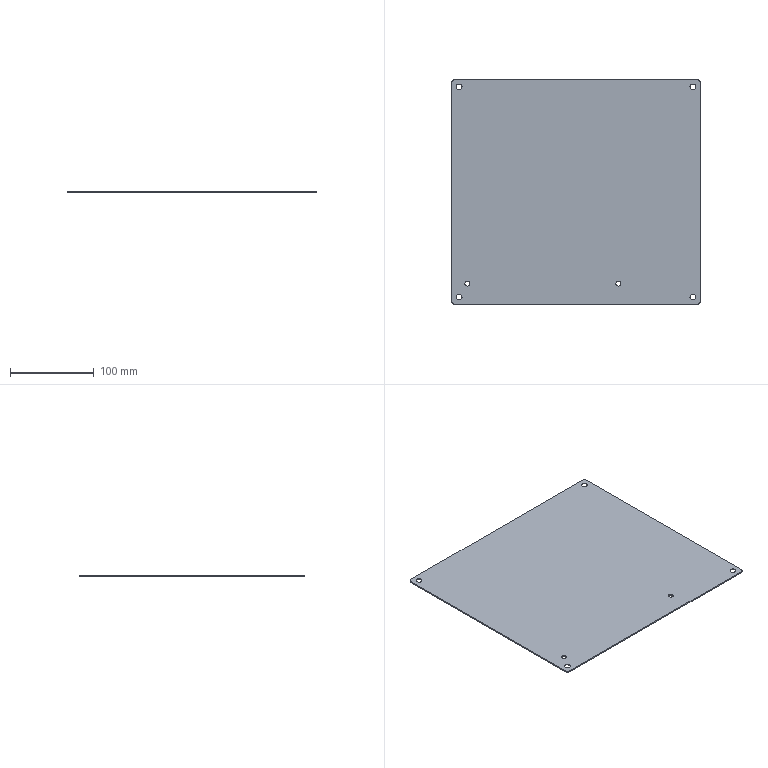Part | SolidWorks | features Chamfer 1, Cut 1, Extrusion 1, Fillet 1, ICE 1 | 1 solid | 30 faces | box 296 x 267.5 x 1.5 mm | volume 118387 mm3 | cylinder 16 | cone 8 | plane 6 | commonest cylinder face diameters 6 x8 7.1 x8
STEP:
#1=CARTESIAN_POINT('',(-94.45,326.,-0.5));
#2=VERTEX_POINT('',#1);
#3=CARTESIAN_POINT('',(-101.55,326.,-0.5));
#4=VERTEX_POINT('',#3);
#5=CARTESIAN_POINT('',(-98.,326.,-0.5));
#6=DIRECTION('',(0.,0.,-1.));
#7=DIRECTION('',(1.,0.,0.));
#8=AXIS2_PLACEMENT_3D('',#5,#6,#7);
#9=CIRCLE('',#8,3.55);
#10=EDGE_CURVE('',#2,#4,#9,.T.);
#11=ORIENTED_EDGE('',*,*,#10,.F.);
#12=CARTESIAN_POINT('',(-93.45,326.,-1.5));
#13=VERTEX_POINT('',#12);
#14=CARTESIAN_POINT('',(-94.45,326.,-0.5));
#15=DIRECTION('',(0.7071,0.,-0.7071));
#16=VECTOR('',#15,1000.);
#17=LINE('',#14,#16);
#18=EDGE_CURVE('',#2,#13,#17,.T.);
#19=ORIENTED_EDGE('',*,*,#18,.T.);
#20=CARTESIAN_POINT('',(-102.55,326.,-1.5));
#21=VERTEX_POINT('',#20);
#22=CARTESIAN_POINT('',(-98.,326.,-1.5));
#23=DIRECTION('',(0.,0.,1.));
#24=DIRECTION('',(1.,0.,0.));
#25=AXIS2_PLACEMENT_3D('',#22,#23,#24);
#26=CIRCLE('',#25,4.55);
#27=EDGE_CURVE('',#21,#13,#26,.T.);
#28=ORIENTED_EDGE('',*,*,#27,.F.);
#29=CARTESIAN_POINT('',(-101.55,326.,-0.5));
#30=DIRECTION('',(-0.7071,0.,-0.7071));
#31=VECTOR('',#30,1000.);
#32=LINE('',#29,#31);
#33=EDGE_CURVE('',#4,#21,#32,.T.);
#34=ORIENTED_EDGE('',*,*,#33,.F.);
#35=EDGE_LOOP('',(#11,#19,#28,#34));
#36=FACE_OUTER_BOUND('',#35,.T.);
#37=CARTESIAN_POINT('',(-98.,326.,-0.5));
#38=DIRECTION('',(0.,0.,-1.));
#39=DIRECTION('',(-1.,0.,0.));
#40=AXIS2_PLACEMENT_3D('',#37,#38,#39);
#41=CONICAL_SURFACE('',#40,3.55,0.7854);
#42=ADVANCED_FACE('',(#36),#41,.F.);
#43=CARTESIAN_POINT('',(-373.45,326.,-0.5));
#44=VERTEX_POINT('',#43);
#45=CARTESIAN_POINT('',(-380.55,326.,-0.5));
#46=VERTEX_POINT('',#45);
#47=CARTESIAN_POINT('',(-377.,326.,-0.5));
#48=DIRECTION('',(0.,0.,-1.));
#49=DIRECTION('',(1.,0.,0.));
#50=AXIS2_PLACEMENT_3D('',#47,#48,#49);
#51=CIRCLE('',#50,3.55);
#52=EDGE_CURVE('',#44,#46,#51,.T.);
#53=ORIENTED_EDGE('',*,*,#52,.F.);
#54=CARTESIAN_POINT('',(-372.45,326.,-1.5));
#55=VERTEX_POINT('',#54);
#56=CARTESIAN_POINT('',(-373.45,326.,-0.5));
#57=DIRECTION('',(0.7071,0.,-0.7071));
#58=VECTOR('',#57,1000.);
#59=LINE('',#56,#58);
#60=EDGE_CURVE('',#44,#55,#59,.T.);
#61=ORIENTED_EDGE('',*,*,#60,.T.);
#62=CARTESIAN_POINT('',(-381.55,326.,-1.5));
#63=VERTEX_POINT('',#62);
#64=CARTESIAN_POINT('',(-377.,326.,-1.5));
#65=DIRECTION('',(0.,0.,1.));
#66=DIRECTION('',(1.,0.,0.));
#67=AXIS2_PLACEMENT_3D('',#64,#65,#66);
#68=CIRCLE('',#67,4.55);
#69=EDGE_CURVE('',#63,#55,#68,.T.);
#70=ORIENTED_EDGE('',*,*,#69,.F.);
#71=CARTESIAN_POINT('',(-380.55,326.,-0.5));
#72=DIRECTION('',(-0.7071,0.,-0.7071));
#73=VECTOR('',#72,1000.);
#74=LINE('',#71,#73);
#75=EDGE_CURVE('',#46,#63,#74,.T.);
#76=ORIENTED_EDGE('',*,*,#75,.F.);
#77=EDGE_LOOP('',(#53,#61,#70,#76));
#78=FACE_OUTER_BOUND('',#77,.T.);
#79=CARTESIAN_POINT('',(-377.,326.,-0.5));
#80=DIRECTION('',(0.,0.,-1.));
#81=DIRECTION('',(-1.,0.,0.));
#82=AXIS2_PLACEMENT_3D('',#79,#80,#81);
#83=CONICAL_SURFACE('',#82,3.55,0.7854);
#84=ADVANCED_FACE('',(#78),#83,.F.);
#85=CARTESIAN_POINT('',(-373.45,75.5,-0.5));
#86=VERTEX_POINT('',#85);
#87=CARTESIAN_POINT('',(-380.55,75.5,-0.5));
#88=VERTEX_POINT('',#87);
#89=CARTESIAN_POINT('',(-377.,75.5,-0.5));
#90=DIRECTION('',(0.,0.,-1.));
#91=DIRECTION('',(1.,0.,0.));
#92=AXIS2_PLACEMENT_3D('',#89,#90,#91);
#93=CIRCLE('',#92,3.55);
#94=EDGE_CURVE('',#86,#88,#93,.T.);
#95=ORIENTED_EDGE('',*,*,#94,.F.);
#96=CARTESIAN_POINT('',(-372.45,75.5,-1.5));
#97=VERTEX_POINT('',#96);
#98=CARTESIAN_POINT('',(-373.45,75.5,-0.5));
#99=DIRECTION('',(0.7071,0.,-0.7071));
#100=VECTOR('',#99,1000.);
#101=LINE('',#98,#100);
#102=EDGE_CURVE('',#86,#97,#101,.T.);
#103=ORIENTED_EDGE('',*,*,#102,.T.);
#104=CARTESIAN_POINT('',(-381.55,75.5,-1.5));
#105=VERTEX_POINT('',#104);
#106=CARTESIAN_POINT('',(-377.,75.5,-1.5));
#107=DIRECTION('',(0.,0.,1.));
#108=DIRECTION('',(1.,0.,0.));
#109=AXIS2_PLACEMENT_3D('',#106,#107,#108);
#110=CIRCLE('',#109,4.55);
#111=EDGE_CURVE('',#105,#97,#110,.T.);
#112=ORIENTED_EDGE('',*,*,#111,.F.);
#113=CARTESIAN_POINT('',(-380.55,75.5,-0.5));
#114=DIRECTION('',(-0.7071,0.,-0.7071));
#115=VECTOR('',#114,1000.);
#116=LINE('',#113,#115);
#117=EDGE_CURVE('',#88,#105,#116,.T.);
#118=ORIENTED_EDGE('',*,*,#117,.F.);
#119=EDGE_LOOP('',(#95,#103,#112,#118));
#120=FACE_OUTER_BOUND('',#119,.T.);
#121=CARTESIAN_POINT('',(-377.,75.5,-0.5));
#122=DIRECTION('',(0.,0.,-1.));
#123=DIRECTION('',(-1.,0.,0.));
#124=AXIS2_PLACEMENT_3D('',#121,#122,#123);
#125=CONICAL_SURFACE('',#124,3.55,0.7854);
#126=ADVANCED_FACE('',(#120),#125,.F.);
#127=CARTESIAN_POINT('',(-94.45,75.5,-0.5));
#128=VERTEX_POINT('',#127);
#129=CARTESIAN_POINT('',(-101.55,75.5,-0.5));
#130=VERTEX_POINT('',#129);
#131=CARTESIAN_POINT('',(-98.,75.5,-0.5));
#132=DIRECTION('',(0.,0.,-1.));
#133=DIRECTION('',(1.,0.,0.));
#134=AXIS2_PLACEMENT_3D('',#131,#132,#133);
#135=CIRCLE('',#134,3.55);
#136=EDGE_CURVE('',#128,#130,#135,.T.);
#137=ORIENTED_EDGE('',*,*,#136,.F.);
#138=CARTESIAN_POINT('',(-93.45,75.5,-1.5));
#139=VERTEX_POINT('',#138);
#140=CARTESIAN_POINT('',(-94.45,75.5,-0.5));
#141=DIRECTION('',(0.7071,0.,-0.7071));
#142=VECTOR('',#141,1000.);
#143=LINE('',#140,#142);
#144=EDGE_CURVE('',#128,#139,#143,.T.);
#145=ORIENTED_EDGE('',*,*,#144,.T.);
#146=CARTESIAN_POINT('',(-102.55,75.5,-1.5));
#147=VERTEX_POINT('',#146);
#148=CARTESIAN_POINT('',(-98.,75.5,-1.5));
#149=DIRECTION('',(0.,0.,1.));
#150=DIRECTION('',(1.,0.,0.));
#151=AXIS2_PLACEMENT_3D('',#148,#149,#150);
#152=CIRCLE('',#151,4.55);
#153=EDGE_CURVE('',#147,#139,#152,.T.);
#154=ORIENTED_EDGE('',*,*,#153,.F.);
#155=CARTESIAN_POINT('',(-101.55,75.5,-0.5));
#156=DIRECTION('',(-0.7071,0.,-0.7071));
#157=VECTOR('',#156,1000.);
#158=LINE('',#155,#157);
#159=EDGE_CURVE('',#130,#147,#158,.T.);
#160=ORIENTED_EDGE('',*,*,#159,.F.);
#161=EDGE_LOOP('',(#137,#145,#154,#160));
#162=FACE_OUTER_BOUND('',#161,.T.);
#163=CARTESIAN_POINT('',(-98.,75.5,-0.5));
#164=DIRECTION('',(0.,0.,-1.));
#165=DIRECTION('',(-1.,0.,0.));
#166=AXIS2_PLACEMENT_3D('',#163,#164,#165);
#167=CONICAL_SURFACE('',#166,3.55,0.7854);
#168=ADVANCED_FACE('',(#162),#167,.F.);
#169=CARTESIAN_POINT('',(-373.45,326.,0.));
#170=VERTEX_POINT('',#169);
#171=CARTESIAN_POINT('',(-380.55,326.,0.));
#172=VERTEX_POINT('',#171);
#173=CARTESIAN_POINT('',(-377.,326.,0.));
#174=DIRECTION('',(0.,0.,-1.));
#175=DIRECTION('',(-1.,0.,0.));
#176=AXIS2_PLACEMENT_3D('',#173,#174,#175);
#177=CIRCLE('',#176,3.55);
#178=EDGE_CURVE('',#170,#172,#177,.T.);
#179=ORIENTED_EDGE('',*,*,#178,.F.);
#180=CARTESIAN_POINT('',(-373.45,326.,0.));
#181=DIRECTION('',(0.,0.,-1.));
#182=VECTOR('',#181,1000.);
#183=LINE('',#180,#182);
#184=EDGE_CURVE('',#170,#44,#183,.T.);
#185=ORIENTED_EDGE('',*,*,#184,.T.);
#186=ORIENTED_EDGE('',*,*,#52,.T.);
#187=CARTESIAN_POINT('',(-380.55,326.,0.));
#188=DIRECTION('',(0.,0.,-1.));
#189=VECTOR('',#188,1000.);
#190=LINE('',#187,#189);
#191=EDGE_CURVE('',#172,#46,#190,.T.);
#192=ORIENTED_EDGE('',*,*,#191,.F.);
#193=EDGE_LOOP('',(#179,#185,#186,#192));
#194=FACE_OUTER_BOUND('',#193,.T.);
#195=CARTESIAN_POINT('',(-377.,326.,0.));
#196=DIRECTION('',(0.,0.,-1.));
#197=DIRECTION('',(-1.,0.,0.));
#198=AXIS2_PLACEMENT_3D('',#195,#196,#197);
#199=CYLINDRICAL_SURFACE('',#198,3.55);
#200=ADVANCED_FACE('',(#194),#199,.F.);
#201=CARTESIAN_POINT('',(-373.45,75.5,0.));
#202=VERTEX_POINT('',#201);
#203=CARTESIAN_POINT('',(-380.55,75.5,0.));
#204=VERTEX_POINT('',#203);
#205=CARTESIAN_POINT('',(-377.,75.5,0.));
#206=DIRECTION('',(0.,0.,-1.));
#207=DIRECTION('',(-1.,0.,0.));
#208=AXIS2_PLACEMENT_3D('',#205,#206,#207);
#209=CIRCLE('',#208,3.55);
#210=EDGE_CURVE('',#202,#204,#209,.T.);
#211=ORIENTED_EDGE('',*,*,#210,.F.);
#212=CARTESIAN_POINT('',(-373.45,75.5,0.));
#213=DIRECTION('',(0.,0.,-1.));
#214=VECTOR('',#213,1000.);
#215=LINE('',#212,#214);
#216=EDGE_CURVE('',#202,#86,#215,.T.);
#217=ORIENTED_EDGE('',*,*,#216,.T.);
#218=ORIENTED_EDGE('',*,*,#94,.T.);
#219=CARTESIAN_POINT('',(-380.55,75.5,0.));
#220=DIRECTION('',(0.,0.,-1.));
#221=VECTOR('',#220,1000.);
#222=LINE('',#219,#221);
#223=EDGE_CURVE('',#204,#88,#222,.T.);
#224=ORIENTED_EDGE('',*,*,#223,.F.);
#225=EDGE_LOOP('',(#211,#217,#218,#224));
#226=FACE_OUTER_BOUND('',#225,.T.);
#227=CARTESIAN_POINT('',(-377.,75.5,0.));
#228=DIRECTION('',(0.,0.,-1.));
#229=DIRECTION('',(-1.,0.,0.));
#230=AXIS2_PLACEMENT_3D('',#227,#228,#229);
#231=CYLINDRICAL_SURFACE('',#230,3.55);
#232=ADVANCED_FACE('',(#226),#231,.F.);
#233=CARTESIAN_POINT('',(-94.45,75.5,0.));
#234=VERTEX_POINT('',#233);
#235=CARTESIAN_POINT('',(-101.55,75.5,0.));
#236=VERTEX_POINT('',#235);
#237=CARTESIAN_POINT('',(-98.,75.5,0.));
#238=DIRECTION('',(0.,0.,-1.));
#239=DIRECTION('',(-1.,0.,0.));
#240=AXIS2_PLACEMENT_3D('',#237,#238,#239);
#241=CIRCLE('',#240,3.55);
#242=EDGE_CURVE('',#234,#236,#241,.T.);
#243=ORIENTED_EDGE('',*,*,#242,.F.);
#244=CARTESIAN_POINT('',(-94.45,75.5,0.));
#245=DIRECTION('',(0.,0.,-1.));
#246=VECTOR('',#245,1000.);
#247=LINE('',#244,#246);
#248=EDGE_CURVE('',#234,#128,#247,.T.);
#249=ORIENTED_EDGE('',*,*,#248,.T.);
#250=ORIENTED_EDGE('',*,*,#136,.T.);
#251=CARTESIAN_POINT('',(-101.55,75.5,0.));
#252=DIRECTION('',(0.,0.,-1.));
#253=VECTOR('',#252,1000.);
#254=LINE('',#251,#253);
#255=EDGE_CURVE('',#236,#130,#254,.T.);
#256=ORIENTED_EDGE('',*,*,#255,.F.);
#257=EDGE_LOOP('',(#243,#249,#250,#256));
#258=FACE_OUTER_BOUND('',#257,.T.);
#259=CARTESIAN_POINT('',(-98.,75.5,0.));
#260=DIRECTION('',(0.,0.,-1.));
#261=DIRECTION('',(-1.,0.,0.));
#262=AXIS2_PLACEMENT_3D('',#259,#260,#261);
#263=CYLINDRICAL_SURFACE('',#262,3.55);
#264=ADVANCED_FACE('',(#258),#263,.F.);
#265=CARTESIAN_POINT('',(-94.45,326.,0.));
#266=VERTEX_POINT('',#265);
#267=CARTESIAN_POINT('',(-101.55,326.,0.));
#268=VERTEX_POINT('',#267);
#269=CARTESIAN_POINT('',(-98.,326.,0.));
#270=DIRECTION('',(0.,0.,-1.));
#271=DIRECTION('',(-1.,0.,0.));
#272=AXIS2_PLACEMENT_3D('',#269,#270,#271);
#273=CIRCLE('',#272,3.55);
#274=EDGE_CURVE('',#266,#268,#273,.T.);
#275=ORIENTED_EDGE('',*,*,#274,.F.);
#276=CARTESIAN_POINT('',(-94.45,326.,0.));
#277=DIRECTION('',(0.,0.,-1.));
#278=VECTOR('',#277,1000.);
#279=LINE('',#276,#278);
#280=EDGE_CURVE('',#266,#2,#279,.T.);
#281=ORIENTED_EDGE('',*,*,#280,.T.);
#282=ORIENTED_EDGE('',*,*,#10,.T.);
#283=CARTESIAN_POINT('',(-101.55,326.,0.));
#284=DIRECTION('',(0.,0.,-1.));
#285=VECTOR('',#284,1000.);
#286=LINE('',#283,#285);
#287=EDGE_CURVE('',#268,#4,#286,.T.);
#288=ORIENTED_EDGE('',*,*,#287,.F.);
#289=EDGE_LOOP('',(#275,#281,#282,#288));
#290=FACE_OUTER_BOUND('',#289,.T.);
#291=CARTESIAN_POINT('',(-98.,326.,0.));
#292=DIRECTION('',(0.,0.,-1.));
#293=DIRECTION('',(-1.,0.,0.));
#294=AXIS2_PLACEMENT_3D('',#291,#292,#293);
#295=CYLINDRICAL_SURFACE('',#294,3.55);
#296=ADVANCED_FACE('',(#290),#295,.F.);
#297=CARTESIAN_POINT('',(-190.,91.5,-1.5));
#298=VERTEX_POINT('',#297);
#299=CARTESIAN_POINT('',(-184.,91.5,-1.5));
#300=VERTEX_POINT('',#299);
#301=CARTESIAN_POINT('',(-187.,91.5,-1.5));
#302=DIRECTION('',(0.,0.,1.));
#303=DIRECTION('',(1.,0.,0.));
#304=AXIS2_PLACEMENT_3D('',#301,#302,#303);
#305=CIRCLE('',#304,3.);
#306=EDGE_CURVE('',#298,#300,#305,.T.);
#307=ORIENTED_EDGE('',*,*,#306,.F.);
#308=CARTESIAN_POINT('',(-190.,91.5,0.));
#309=VERTEX_POINT('',#308);
#310=CARTESIAN_POINT('',(-190.,91.5,-1.5));
#311=DIRECTION('',(0.,0.,1.));
#312=VECTOR('',#311,1000.);
#313=LINE('',#310,#312);
#314=EDGE_CURVE('',#298,#309,#313,.T.);
#315=ORIENTED_EDGE('',*,*,#314,.T.);
#316=CARTESIAN_POINT('',(-184.,91.5,0.));
#317=VERTEX_POINT('',#316);
#318=CARTESIAN_POINT('',(-187.,91.5,0.));
#319=DIRECTION('',(0.,0.,1.));
#320=DIRECTION('',(1.,0.,0.));
#321=AXIS2_PLACEMENT_3D('',#318,#319,#320);
#322=CIRCLE('',#321,3.);
#323=EDGE_CURVE('',#309,#317,#322,.T.);
#324=ORIENTED_EDGE('',*,*,#323,.T.);
#325=CARTESIAN_POINT('',(-184.,91.5,-1.5));
#326=DIRECTION('',(0.,0.,1.));
#327=VECTOR('',#326,1000.);
#328=LINE('',#325,#327);
#329=EDGE_CURVE('',#300,#317,#328,.T.);
#330=ORIENTED_EDGE('',*,*,#329,.F.);
#331=EDGE_LOOP('',(#307,#315,#324,#330));
#332=FACE_OUTER_BOUND('',#331,.T.);
#333=CARTESIAN_POINT('',(-187.,91.5,-1.5));
#334=DIRECTION('',(0.,0.,1.));
#335=DIRECTION('',(1.,0.,0.));
#336=AXIS2_PLACEMENT_3D('',#333,#334,#335);
#337=CYLINDRICAL_SURFACE('',#336,3.);
#338=ADVANCED_FACE('',(#332),#337,.F.);
#339=CARTESIAN_POINT('',(-370.,91.5,-1.5));
#340=VERTEX_POINT('',#339);
#341=CARTESIAN_POINT('',(-364.,91.5,-1.5));
#342=VERTEX_POINT('',#341);
#343=CARTESIAN_POINT('',(-367.,91.5,-1.5));
#344=DIRECTION('',(0.,0.,1.));
#345=DIRECTION('',(1.,0.,0.));
#346=AXIS2_PLACEMENT_3D('',#343,#344,#345);
#347=CIRCLE('',#346,3.);
#348=EDGE_CURVE('',#340,#342,#347,.T.);
#349=ORIENTED_EDGE('',*,*,#348,.F.);
#350=CARTESIAN_POINT('',(-370.,91.5,0.));
#351=VERTEX_POINT('',#350);
#352=CARTESIAN_POINT('',(-370.,91.5,-1.5));
#353=DIRECTION('',(0.,0.,1.));
#354=VECTOR('',#353,1000.);
#355=LINE('',#352,#354);
#356=EDGE_CURVE('',#340,#351,#355,.T.);
#357=ORIENTED_EDGE('',*,*,#356,.T.);
#358=CARTESIAN_POINT('',(-364.,91.5,0.));
#359=VERTEX_POINT('',#358);
#360=CARTESIAN_POINT('',(-367.,91.5,0.));
#361=DIRECTION('',(0.,0.,1.));
#362=DIRECTION('',(1.,0.,0.));
#363=AXIS2_PLACEMENT_3D('',#360,#361,#362);
#364=CIRCLE('',#363,3.);
#365=EDGE_CURVE('',#351,#359,#364,.T.);
#366=ORIENTED_EDGE('',*,*,#365,.T.);
#367=CARTESIAN_POINT('',(-364.,91.5,-1.5));
#368=DIRECTION('',(0.,0.,1.));
#369=VECTOR('',#368,1000.);
#370=LINE('',#367,#369);
#371=EDGE_CURVE('',#342,#359,#370,.T.);
#372=ORIENTED_EDGE('',*,*,#371,.F.);
#373=EDGE_LOOP('',(#349,#357,#366,#372));
#374=FACE_OUTER_BOUND('',#373,.T.);
#375=CARTESIAN_POINT('',(-367.,91.5,-1.5));
#376=DIRECTION('',(0.,0.,1.));
#377=DIRECTION('',(1.,0.,0.));
#378=AXIS2_PLACEMENT_3D('',#375,#376,#377);
#379=CYLINDRICAL_SURFACE('',#378,3.);
#380=ADVANCED_FACE('',(#374),#379,.F.);
#381=CARTESIAN_POINT('',(-382.5,67.,-1.5));
#382=VERTEX_POINT('',#381);
#383=CARTESIAN_POINT('',(-92.5,67.,-1.5));
#384=VERTEX_POINT('',#383);
#385=CARTESIAN_POINT('',(-385.5,67.,-1.5));
#386=DIRECTION('',(1.,0.,0.));
#387=VECTOR('',#386,1000.);
#388=LINE('',#385,#387);
#389=EDGE_CURVE('',#382,#384,#388,.T.);
#390=ORIENTED_EDGE('',*,*,#389,.T.);
#391=CARTESIAN_POINT('',(-92.5,67.,0.));
#392=VERTEX_POINT('',#391);
#393=CARTESIAN_POINT('',(-92.5,67.,-1.5));
#394=DIRECTION('',(0.,0.,1.));
#395=VECTOR('',#394,1000.);
#396=LINE('',#393,#395);
#397=EDGE_CURVE('',#384,#392,#396,.T.);
#398=ORIENTED_EDGE('',*,*,#397,.T.);
#399=CARTESIAN_POINT('',(-382.5,67.,0.));
#400=VERTEX_POINT('',#399);
#401=CARTESIAN_POINT('',(-385.5,67.,0.));
#402=DIRECTION('',(1.,0.,0.));
#403=VECTOR('',#402,1000.);
#404=LINE('',#401,#403);
#405=EDGE_CURVE('',#400,#392,#404,.T.);
#406=ORIENTED_EDGE('',*,*,#405,.F.);
#407=CARTESIAN_POINT('',(-382.5,67.,-1.5));
#408=DIRECTION('',(0.,0.,-1.));
#409=VECTOR('',#408,1000.);
#410=LINE('',#407,#409);
#411=EDGE_CURVE('',#400,#382,#410,.T.);
#412=ORIENTED_EDGE('',*,*,#411,.T.);
#413=EDGE_LOOP('',(#390,#398,#406,#412));
#414=FACE_OUTER_BOUND('',#413,.T.);
#415=CARTESIAN_POINT('',(-385.5,67.,-1.5));
#416=DIRECTION('',(0.,-1.,0.));
#417=DIRECTION('',(0.,0.,-1.));
#418=AXIS2_PLACEMENT_3D('',#415,#416,#417);
#419=PLANE('',#418);
#420=ADVANCED_FACE('',(#414),#419,.T.);
#421=CARTESIAN_POINT('',(-385.5,331.5,-1.5));
#422=VERTEX_POINT('',#421);
#423=CARTESIAN_POINT('',(-385.5,70.,-1.5));
#424=VERTEX_POINT('',#423);
#425=CARTESIAN_POINT('',(-385.5,334.5,-1.5));
#426=DIRECTION('',(0.,-1.,0.));
#427=VECTOR('',#426,1000.);
#428=LINE('',#425,#427);
#429=EDGE_CURVE('',#422,#424,#428,.T.);
#430=ORIENTED_EDGE('',*,*,#429,.T.);
#431=CARTESIAN_POINT('',(-385.5,70.,0.));
#432=VERTEX_POINT('',#431);
#433=CARTESIAN_POINT('',(-385.5,70.,-1.5));
#434=DIRECTION('',(0.,0.,1.));
#435=VECTOR('',#434,1000.);
#436=LINE('',#433,#435);
#437=EDGE_CURVE('',#424,#432,#436,.T.);
#438=ORIENTED_EDGE('',*,*,#437,.T.);
#439=CARTESIAN_POINT('',(-385.5,331.5,0.));
#440=VERTEX_POINT('',#439);
#441=CARTESIAN_POINT('',(-385.5,334.5,0.));
#442=DIRECTION('',(0.,-1.,0.));
#443=VECTOR('',#442,1000.);
#444=LINE('',#441,#443);
#445=EDGE_CURVE('',#440,#432,#444,.T.);
#446=ORIENTED_EDGE('',*,*,#445,.F.);
#447=CARTESIAN_POINT('',(-385.5,331.5,-1.5));
#448=DIRECTION('',(0.,0.,-1.));
#449=VECTOR('',#448,1000.);
#450=LINE('',#447,#449);
#451=EDGE_CURVE('',#440,#422,#450,.T.);
#452=ORIENTED_EDGE('',*,*,#451,.T.);
#453=EDGE_LOOP('',(#430,#438,#446,#452));
#454=FACE_OUTER_BOUND('',#453,.T.);
#455=CARTESIAN_POINT('',(-385.5,334.5,-1.5));
#456=DIRECTION('',(-1.,0.,0.));
#457=DIRECTION('',(0.,-1.,0.));
#458=AXIS2_PLACEMENT_3D('',#455,#456,#457);
#459=PLANE('',#458);
#460=ADVANCED_FACE('',(#454),#459,.T.);
#461=CARTESIAN_POINT('',(-92.5,334.5,0.));
#462=VERTEX_POINT('',#461);
#463=CARTESIAN_POINT('',(-382.5,334.5,0.));
#464=VERTEX_POINT('',#463);
#465=CARTESIAN_POINT('',(-89.5,334.5,0.));
#466=DIRECTION('',(-1.,0.,0.));
#467=VECTOR('',#466,1000.);
#468=LINE('',#465,#467);
#469=EDGE_CURVE('',#462,#464,#468,.T.);
#470=ORIENTED_EDGE('',*,*,#469,.F.);
#471=CARTESIAN_POINT('',(-92.5,334.5,-1.5));
#472=VERTEX_POINT('',#471);
#473=CARTESIAN_POINT('',(-92.5,334.5,-1.5));
#474=DIRECTION('',(0.,0.,-1.));
#475=VECTOR('',#474,1000.);
#476=LINE('',#473,#475);
#477=EDGE_CURVE('',#462,#472,#476,.T.);
#478=ORIENTED_EDGE('',*,*,#477,.T.);
#479=CARTESIAN_POINT('',(-382.5,334.5,-1.5));
#480=VERTEX_POINT('',#479);
#481=CARTESIAN_POINT('',(-89.5,334.5,-1.5));
#482=DIRECTION('',(-1.,0.,0.));
#483=VECTOR('',#482,1000.);
#484=LINE('',#481,#483);
#485=EDGE_CURVE('',#472,#480,#484,.T.);
#486=ORIENTED_EDGE('',*,*,#485,.T.);
#487=CARTESIAN_POINT('',(-382.5,334.5,-1.5));
#488=DIRECTION('',(0.,0.,1.));
#489=VECTOR('',#488,1000.);
#490=LINE('',#487,#489);
#491=EDGE_CURVE('',#480,#464,#490,.T.);
#492=ORIENTED_EDGE('',*,*,#491,.T.);
#493=EDGE_LOOP('',(#470,#478,#486,#492));
#494=FACE_OUTER_BOUND('',#493,.T.);
#495=CARTESIAN_POINT('',(-89.5,334.5,-1.5));
#496=DIRECTION('',(0.,1.,0.));
#497=DIRECTION('',(0.,0.,1.));
#498=AXIS2_PLACEMENT_3D('',#495,#496,#497);
#499=PLANE('',#498);
#500=ADVANCED_FACE('',(#494),#499,.T.);
#501=CARTESIAN_POINT('',(-89.5,70.,0.));
#502=VERTEX_POINT('',#501);
#503=CARTESIAN_POINT('',(-89.5,331.5,0.));
#504=VERTEX_POINT('',#503);
#505=CARTESIAN_POINT('',(-89.5,67.,0.));
#506=DIRECTION('',(0.,1.,0.));
#507=VECTOR('',#506,1000.);
#508=LINE('',#505,#507);
#509=EDGE_CURVE('',#502,#504,#508,.T.);
#510=ORIENTED_EDGE('',*,*,#509,.F.);
#511=CARTESIAN_POINT('',(-89.5,70.,-1.5));
#512=VERTEX_POINT('',#511);
#513=CARTESIAN_POINT('',(-89.5,70.,-1.5));
#514=DIRECTION('',(0.,0.,-1.));
#515=VECTOR('',#514,1000.);
#516=LINE('',#513,#515);
#517=EDGE_CURVE('',#502,#512,#516,.T.);
#518=ORIENTED_EDGE('',*,*,#517,.T.);
#519=CARTESIAN_POINT('',(-89.5,331.5,-1.5));
#520=VERTEX_POINT('',#519);
#521=CARTESIAN_POINT('',(-89.5,67.,-1.5));
#522=DIRECTION('',(0.,1.,0.));
#523=VECTOR('',#522,1000.);
#524=LINE('',#521,#523);
#525=EDGE_CURVE('',#512,#520,#524,.T.);
#526=ORIENTED_EDGE('',*,*,#525,.T.);
#527=CARTESIAN_POINT('',(-89.5,331.5,-1.5));
#528=DIRECTION('',(0.,0.,1.));
#529=VECTOR('',#528,1000.);
#530=LINE('',#527,#529);
#531=EDGE_CURVE('',#520,#504,#530,.T.);
#532=ORIENTED_EDGE('',*,*,#531,.T.);
#533=EDGE_LOOP('',(#510,#518,#526,#532));
#534=FACE_OUTER_BOUND('',#533,.T.);
#535=CARTESIAN_POINT('',(-89.5,67.,-1.5));
#536=DIRECTION('',(1.,0.,0.));
#537=DIRECTION('',(0.,1.,0.));
#538=AXIS2_PLACEMENT_3D('',#535,#536,#537);
#539=PLANE('',#538);
#540=ADVANCED_FACE('',(#534),#539,.T.);
#541=ORIENTED_EDGE('',*,*,#153,.T.);
#542=CARTESIAN_POINT('',(-98.,75.5,-1.5));
#543=DIRECTION('',(0.,0.,1.));
#544=DIRECTION('',(1.,0.,0.));
#545=AXIS2_PLACEMENT_3D('',#542,#543,#544);
#546=CIRCLE('',#545,4.55);
#547=EDGE_CURVE('',#139,#147,#546,.T.);
#548=ORIENTED_EDGE('',*,*,#547,.T.);
#549=EDGE_LOOP('',(#541,#548));
#550=FACE_BOUND('',#549,.T.);
#551=ORIENTED_EDGE('',*,*,#111,.T.);
#552=CARTESIAN_POINT('',(-377.,75.5,-1.5));
#553=DIRECTION('',(0.,0.,1.));
#554=DIRECTION('',(1.,0.,0.));
#555=AXIS2_PLACEMENT_3D('',#552,#553,#554);
#556=CIRCLE('',#555,4.55);
#557=EDGE_CURVE('',#97,#105,#556,.T.);
#558=ORIENTED_EDGE('',*,*,#557,.T.);
#559=EDGE_LOOP('',(#551,#558));
#560=FACE_BOUND('',#559,.T.);
#561=ORIENTED_EDGE('',*,*,#69,.T.);
#562=CARTESIAN_POINT('',(-377.,326.,-1.5));
#563=DIRECTION('',(0.,0.,1.));
#564=DIRECTION('',(1.,0.,0.));
#565=AXIS2_PLACEMENT_3D('',#562,#563,#564);
#566=CIRCLE('',#565,4.55);
#567=EDGE_CURVE('',#55,#63,#566,.T.);
#568=ORIENTED_EDGE('',*,*,#567,.T.);
#569=EDGE_LOOP('',(#561,#568));
#570=FACE_BOUND('',#569,.T.);
#571=ORIENTED_EDGE('',*,*,#27,.T.);
#572=CARTESIAN_POINT('',(-98.,326.,-1.5));
#573=DIRECTION('',(0.,0.,1.));
#574=DIRECTION('',(1.,0.,0.));
#575=AXIS2_PLACEMENT_3D('',#572,#573,#574);
#576=CIRCLE('',#575,4.55);
#577=EDGE_CURVE('',#13,#21,#576,.T.);
#578=ORIENTED_EDGE('',*,*,#577,.T.);
#579=EDGE_LOOP('',(#571,#578));
#580=FACE_BOUND('',#579,.T.);
#581=CARTESIAN_POINT('',(-187.,91.5,-1.5));
#582=DIRECTION('',(0.,0.,1.));
#583=DIRECTION('',(1.,0.,0.));
#584=AXIS2_PLACEMENT_3D('',#581,#582,#583);
#585=CIRCLE('',#584,3.);
#586=EDGE_CURVE('',#300,#298,#585,.T.);
#587=ORIENTED_EDGE('',*,*,#586,.T.);
#588=ORIENTED_EDGE('',*,*,#306,.T.);
#589=EDGE_LOOP('',(#587,#588));
#590=FACE_BOUND('',#589,.T.);
#591=CARTESIAN_POINT('',(-367.,91.5,-1.5));
#592=DIRECTION('',(0.,0.,1.));
#593=DIRECTION('',(1.,0.,0.));
#594=AXIS2_PLACEMENT_3D('',#591,#592,#593);
#595=CIRCLE('',#594,3.);
#596=EDGE_CURVE('',#342,#340,#595,.T.);
#597=ORIENTED_EDGE('',*,*,#596,.T.);
#598=ORIENTED_EDGE('',*,*,#348,.T.);
#599=EDGE_LOOP('',(#597,#598));
#600=FACE_BOUND('',#599,.T.);
#601=ORIENTED_EDGE('',*,*,#525,.F.);
#602=CARTESIAN_POINT('',(-92.5,70.,-1.5));
#603=DIRECTION('',(0.,0.,-1.));
#604=DIRECTION('',(1.,0.,0.));
#605=AXIS2_PLACEMENT_3D('',#602,#603,#604);
#606=CIRCLE('',#605,3.);
#607=EDGE_CURVE('',#512,#384,#606,.T.);
#608=ORIENTED_EDGE('',*,*,#607,.T.);
#609=ORIENTED_EDGE('',*,*,#389,.F.);
#610=CARTESIAN_POINT('',(-382.5,70.,-1.5));
#611=DIRECTION('',(0.,0.,-1.));
#612=DIRECTION('',(1.,0.,0.));
#613=AXIS2_PLACEMENT_3D('',#610,#611,#612);
#614=CIRCLE('',#613,3.);
#615=EDGE_CURVE('',#382,#424,#614,.T.);
#616=ORIENTED_EDGE('',*,*,#615,.T.);
#617=ORIENTED_EDGE('',*,*,#429,.F.);
#618=CARTESIAN_POINT('',(-382.5,331.5,-1.5));
#619=DIRECTION('',(0.,0.,-1.));
#620=DIRECTION('',(1.,0.,0.));
#621=AXIS2_PLACEMENT_3D('',#618,#619,#620);
#622=CIRCLE('',#621,3.);
#623=EDGE_CURVE('',#422,#480,#622,.T.);
#624=ORIENTED_EDGE('',*,*,#623,.T.);
#625=ORIENTED_EDGE('',*,*,#485,.F.);
#626=CARTESIAN_POINT('',(-92.5,331.5,-1.5));
#627=DIRECTION('',(0.,0.,-1.));
#628=DIRECTION('',(1.,0.,0.));
#629=AXIS2_PLACEMENT_3D('',#626,#627,#628);
#630=CIRCLE('',#629,3.);
#631=EDGE_CURVE('',#472,#520,#630,.T.);
#632=ORIENTED_EDGE('',*,*,#631,.T.);
#633=EDGE_LOOP('',(#601,#608,#609,#616,#617,#624,#625,#632));
#634=FACE_OUTER_BOUND('',#633,.T.);
#635=CARTESIAN_POINT('',(0.,0.,-1.5));
#636=DIRECTION('',(0.,0.,1.));
#637=DIRECTION('',(1.,0.,0.));
#638=AXIS2_PLACEMENT_3D('',#635,#636,#637);
#639=PLANE('',#638);
#640=ADVANCED_FACE('',(#550,#560,#570,#580,#590,#600,#634),#639,.F.);
#641=CARTESIAN_POINT('',(-377.,326.,0.));
#642=DIRECTION('',(0.,0.,-1.));
#643=DIRECTION('',(-1.,0.,0.));
#644=AXIS2_PLACEMENT_3D('',#641,#642,#643);
#645=CIRCLE('',#644,3.55);
#646=EDGE_CURVE('',#172,#170,#645,.T.);
#647=ORIENTED_EDGE('',*,*,#646,.T.);
#648=ORIENTED_EDGE('',*,*,#178,.T.);
#649=EDGE_LOOP('',(#647,#648));
#650=FACE_BOUND('',#649,.T.);
#651=CARTESIAN_POINT('',(-377.,75.5,0.));
#652=DIRECTION('',(0.,0.,-1.));
#653=DIRECTION('',(-1.,0.,0.));
#654=AXIS2_PLACEMENT_3D('',#651,#652,#653);
#655=CIRCLE('',#654,3.55);
#656=EDGE_CURVE('',#204,#202,#655,.T.);
#657=ORIENTED_EDGE('',*,*,#656,.T.);
#658=ORIENTED_EDGE('',*,*,#210,.T.);
#659=EDGE_LOOP('',(#657,#658));
#660=FACE_BOUND('',#659,.T.);
#661=CARTESIAN_POINT('',(-98.,75.5,0.));
#662=DIRECTION('',(0.,0.,-1.));
#663=DIRECTION('',(-1.,0.,0.));
#664=AXIS2_PLACEMENT_3D('',#661,#662,#663);
#665=CIRCLE('',#664,3.55);
#666=EDGE_CURVE('',#236,#234,#665,.T.);
#667=ORIENTED_EDGE('',*,*,#666,.T.);
#668=ORIENTED_EDGE('',*,*,#242,.T.);
#669=EDGE_LOOP('',(#667,#668));
#670=FACE_BOUND('',#669,.T.);
#671=CARTESIAN_POINT('',(-98.,326.,0.));
#672=DIRECTION('',(0.,0.,-1.));
#673=DIRECTION('',(-1.,0.,0.));
#674=AXIS2_PLACEMENT_3D('',#671,#672,#673);
#675=CIRCLE('',#674,3.55);
#676=EDGE_CURVE('',#268,#266,#675,.T.);
#677=ORIENTED_EDGE('',*,*,#676,.T.);
#678=ORIENTED_EDGE('',*,*,#274,.T.);
#679=EDGE_LOOP('',(#677,#678));
#680=FACE_BOUND('',#679,.T.);
#681=CARTESIAN_POINT('',(-187.,91.5,0.));
#682=DIRECTION('',(0.,0.,1.));
#683=DIRECTION('',(1.,0.,0.));
#684=AXIS2_PLACEMENT_3D('',#681,#682,#683);
#685=CIRCLE('',#684,3.);
#686=EDGE_CURVE('',#317,#309,#685,.T.);
#687=ORIENTED_EDGE('',*,*,#686,.F.);
#688=ORIENTED_EDGE('',*,*,#323,.F.);
#689=EDGE_LOOP('',(#687,#688));
#690=FACE_BOUND('',#689,.T.);
#691=CARTESIAN_POINT('',(-367.,91.5,0.));
#692=DIRECTION('',(0.,0.,1.));
#693=DIRECTION('',(1.,0.,0.));
#694=AXIS2_PLACEMENT_3D('',#691,#692,#693);
#695=CIRCLE('',#694,3.);
#696=EDGE_CURVE('',#359,#351,#695,.T.);
#697=ORIENTED_EDGE('',*,*,#696,.F.);
#698=ORIENTED_EDGE('',*,*,#365,.F.);
#699=EDGE_LOOP('',(#697,#698));
#700=FACE_BOUND('',#699,.T.);
#701=ORIENTED_EDGE('',*,*,#405,.T.);
#702=CARTESIAN_POINT('',(-92.5,70.,0.));
#703=DIRECTION('',(0.,0.,1.));
#704=DIRECTION('',(1.,0.,0.));
#705=AXIS2_PLACEMENT_3D('',#702,#703,#704);
#706=CIRCLE('',#705,3.);
#707=EDGE_CURVE('',#392,#502,#706,.T.);
#708=ORIENTED_EDGE('',*,*,#707,.T.);
#709=ORIENTED_EDGE('',*,*,#509,.T.);
#710=CARTESIAN_POINT('',(-92.5,331.5,0.));
#711=DIRECTION('',(0.,0.,1.));
#712=DIRECTION('',(1.,0.,0.));
#713=AXIS2_PLACEMENT_3D('',#710,#711,#712);
#714=CIRCLE('',#713,3.);
#715=EDGE_CURVE('',#504,#462,#714,.T.);
#716=ORIENTED_EDGE('',*,*,#715,.T.);
#717=ORIENTED_EDGE('',*,*,#469,.T.);
#718=CARTESIAN_POINT('',(-382.5,331.5,0.));
#719=DIRECTION('',(0.,0.,1.));
#720=DIRECTION('',(1.,0.,0.));
#721=AXIS2_PLACEMENT_3D('',#718,#719,#720);
#722=CIRCLE('',#721,3.);
#723=EDGE_CURVE('',#464,#440,#722,.T.);
#724=ORIENTED_EDGE('',*,*,#723,.T.);
#725=ORIENTED_EDGE('',*,*,#445,.T.);
#726=CARTESIAN_POINT('',(-382.5,70.,0.));
#727=DIRECTION('',(0.,0.,1.));
#728=DIRECTION('',(1.,0.,0.));
#729=AXIS2_PLACEMENT_3D('',#726,#727,#728);
#730=CIRCLE('',#729,3.);
#731=EDGE_CURVE('',#432,#400,#730,.T.);
#732=ORIENTED_EDGE('',*,*,#731,.T.);
#733=EDGE_LOOP('',(#701,#708,#709,#716,#717,#724,#725,#732));
#734=FACE_OUTER_BOUND('',#733,.T.);
#735=CARTESIAN_POINT('',(0.,0.,0.));
#736=DIRECTION('',(0.,0.,1.));
#737=DIRECTION('',(1.,0.,0.));
#738=AXIS2_PLACEMENT_3D('',#735,#736,#737);
#739=PLANE('',#738);
#740=ADVANCED_FACE('',(#650,#660,#670,#680,#690,#700,#734),#739,.T.);
#741=ORIENTED_EDGE('',*,*,#607,.F.);
#742=ORIENTED_EDGE('',*,*,#517,.F.);
#743=ORIENTED_EDGE('',*,*,#707,.F.);
#744=ORIENTED_EDGE('',*,*,#397,.F.);
#745=EDGE_LOOP('',(#741,#742,#743,#744));
#746=FACE_OUTER_BOUND('',#745,.T.);
#747=CARTESIAN_POINT('',(-92.5,70.,-1.5));
#748=DIRECTION('',(0.,0.,1.));
#749=DIRECTION('',(1.,0.,0.));
#750=AXIS2_PLACEMENT_3D('',#747,#748,#749);
#751=CYLINDRICAL_SURFACE('',#750,3.);
#752=ADVANCED_FACE('',(#746),#751,.T.);
#753=ORIENTED_EDGE('',*,*,#631,.F.);
#754=ORIENTED_EDGE('',*,*,#477,.F.);
#755=ORIENTED_EDGE('',*,*,#715,.F.);
#756=ORIENTED_EDGE('',*,*,#531,.F.);
#757=EDGE_LOOP('',(#753,#754,#755,#756));
#758=FACE_OUTER_BOUND('',#757,.T.);
#759=CARTESIAN_POINT('',(-92.5,331.5,-1.5));
#760=DIRECTION('',(0.,0.,1.));
#761=DIRECTION('',(1.,0.,0.));
#762=AXIS2_PLACEMENT_3D('',#759,#760,#761);
#763=CYLINDRICAL_SURFACE('',#762,3.);
#764=ADVANCED_FACE('',(#758),#763,.T.);
#765=ORIENTED_EDGE('',*,*,#615,.F.);
#766=ORIENTED_EDGE('',*,*,#411,.F.);
#767=ORIENTED_EDGE('',*,*,#731,.F.);
#768=ORIENTED_EDGE('',*,*,#437,.F.);
#769=EDGE_LOOP('',(#765,#766,#767,#768));
#770=FACE_OUTER_BOUND('',#769,.T.);
#771=CARTESIAN_POINT('',(-382.5,70.,-1.5));
#772=DIRECTION('',(0.,0.,1.));
#773=DIRECTION('',(1.,0.,0.));
#774=AXIS2_PLACEMENT_3D('',#771,#772,#773);
#775=CYLINDRICAL_SURFACE('',#774,3.);
#776=ADVANCED_FACE('',(#770),#775,.T.);
#777=ORIENTED_EDGE('',*,*,#623,.F.);
#778=ORIENTED_EDGE('',*,*,#451,.F.);
#779=ORIENTED_EDGE('',*,*,#723,.F.);
#780=ORIENTED_EDGE('',*,*,#491,.F.);
#781=EDGE_LOOP('',(#777,#778,#779,#780));
#782=FACE_OUTER_BOUND('',#781,.T.);
#783=CARTESIAN_POINT('',(-382.5,331.5,-1.5));
#784=DIRECTION('',(0.,0.,1.));
#785=DIRECTION('',(1.,0.,0.));
#786=AXIS2_PLACEMENT_3D('',#783,#784,#785);
#787=CYLINDRICAL_SURFACE('',#786,3.);
#788=ADVANCED_FACE('',(#782),#787,.T.);
#789=ORIENTED_EDGE('',*,*,#356,.F.);
#790=ORIENTED_EDGE('',*,*,#596,.F.);
#791=ORIENTED_EDGE('',*,*,#371,.T.);
#792=ORIENTED_EDGE('',*,*,#696,.T.);
#793=EDGE_LOOP('',(#789,#790,#791,#792));
#794=FACE_OUTER_BOUND('',#793,.T.);
#795=CARTESIAN_POINT('',(-367.,91.5,-1.5));
#796=DIRECTION('',(0.,0.,1.));
#797=DIRECTION('',(1.,0.,0.));
#798=AXIS2_PLACEMENT_3D('',#795,#796,#797);
#799=CYLINDRICAL_SURFACE('',#798,3.);
#800=ADVANCED_FACE('',(#794),#799,.F.);
#801=ORIENTED_EDGE('',*,*,#314,.F.);
#802=ORIENTED_EDGE('',*,*,#586,.F.);
#803=ORIENTED_EDGE('',*,*,#329,.T.);
#804=ORIENTED_EDGE('',*,*,#686,.T.);
#805=EDGE_LOOP('',(#801,#802,#803,#804));
#806=FACE_OUTER_BOUND('',#805,.T.);
#807=CARTESIAN_POINT('',(-187.,91.5,-1.5));
#808=DIRECTION('',(0.,0.,1.));
#809=DIRECTION('',(1.,0.,0.));
#810=AXIS2_PLACEMENT_3D('',#807,#808,#809);
#811=CYLINDRICAL_SURFACE('',#810,3.);
#812=ADVANCED_FACE('',(#806),#811,.F.);
#813=ORIENTED_EDGE('',*,*,#280,.F.);
#814=ORIENTED_EDGE('',*,*,#676,.F.);
#815=ORIENTED_EDGE('',*,*,#287,.T.);
#816=CARTESIAN_POINT('',(-98.,326.,-0.5));
#817=DIRECTION('',(0.,0.,-1.));
#818=DIRECTION('',(1.,0.,0.));
#819=AXIS2_PLACEMENT_3D('',#816,#817,#818);
#820=CIRCLE('',#819,3.55);
#821=EDGE_CURVE('',#4,#2,#820,.T.);
#822=ORIENTED_EDGE('',*,*,#821,.T.);
#823=EDGE_LOOP('',(#813,#814,#815,#822));
#824=FACE_OUTER_BOUND('',#823,.T.);
#825=CARTESIAN_POINT('',(-98.,326.,0.));
#826=DIRECTION('',(0.,0.,-1.));
#827=DIRECTION('',(-1.,0.,0.));
#828=AXIS2_PLACEMENT_3D('',#825,#826,#827);
#829=CYLINDRICAL_SURFACE('',#828,3.55);
#830=ADVANCED_FACE('',(#824),#829,.F.);
#831=ORIENTED_EDGE('',*,*,#248,.F.);
#832=ORIENTED_EDGE('',*,*,#666,.F.);
#833=ORIENTED_EDGE('',*,*,#255,.T.);
#834=CARTESIAN_POINT('',(-98.,75.5,-0.5));
#835=DIRECTION('',(0.,0.,-1.));
#836=DIRECTION('',(1.,0.,0.));
#837=AXIS2_PLACEMENT_3D('',#834,#835,#836);
#838=CIRCLE('',#837,3.55);
#839=EDGE_CURVE('',#130,#128,#838,.T.);
#840=ORIENTED_EDGE('',*,*,#839,.T.);
#841=EDGE_LOOP('',(#831,#832,#833,#840));
#842=FACE_OUTER_BOUND('',#841,.T.);
#843=CARTESIAN_POINT('',(-98.,75.5,0.));
#844=DIRECTION('',(0.,0.,-1.));
#845=DIRECTION('',(-1.,0.,0.));
#846=AXIS2_PLACEMENT_3D('',#843,#844,#845);
#847=CYLINDRICAL_SURFACE('',#846,3.55);
#848=ADVANCED_FACE('',(#842),#847,.F.);
#849=ORIENTED_EDGE('',*,*,#216,.F.);
#850=ORIENTED_EDGE('',*,*,#656,.F.);
#851=ORIENTED_EDGE('',*,*,#223,.T.);
#852=CARTESIAN_POINT('',(-377.,75.5,-0.5));
#853=DIRECTION('',(0.,0.,-1.));
#854=DIRECTION('',(1.,0.,0.));
#855=AXIS2_PLACEMENT_3D('',#852,#853,#854);
#856=CIRCLE('',#855,3.55);
#857=EDGE_CURVE('',#88,#86,#856,.T.);
#858=ORIENTED_EDGE('',*,*,#857,.T.);
#859=EDGE_LOOP('',(#849,#850,#851,#858));
#860=FACE_OUTER_BOUND('',#859,.T.);
#861=CARTESIAN_POINT('',(-377.,75.5,0.));
#862=DIRECTION('',(0.,0.,-1.));
#863=DIRECTION('',(-1.,0.,0.));
#864=AXIS2_PLACEMENT_3D('',#861,#862,#863);
#865=CYLINDRICAL_SURFACE('',#864,3.55);
#866=ADVANCED_FACE('',(#860),#865,.F.);
#867=ORIENTED_EDGE('',*,*,#184,.F.);
#868=ORIENTED_EDGE('',*,*,#646,.F.);
#869=ORIENTED_EDGE('',*,*,#191,.T.);
#870=CARTESIAN_POINT('',(-377.,326.,-0.5));
#871=DIRECTION('',(0.,0.,-1.));
#872=DIRECTION('',(1.,0.,0.));
#873=AXIS2_PLACEMENT_3D('',#870,#871,#872);
#874=CIRCLE('',#873,3.55);
#875=EDGE_CURVE('',#46,#44,#874,.T.);
#876=ORIENTED_EDGE('',*,*,#875,.T.);
#877=EDGE_LOOP('',(#867,#868,#869,#876));
#878=FACE_OUTER_BOUND('',#877,.T.);
#879=CARTESIAN_POINT('',(-377.,326.,0.));
#880=DIRECTION('',(0.,0.,-1.));
#881=DIRECTION('',(-1.,0.,0.));
#882=AXIS2_PLACEMENT_3D('',#879,#880,#881);
#883=CYLINDRICAL_SURFACE('',#882,3.55);
#884=ADVANCED_FACE('',(#878),#883,.F.);
#885=ORIENTED_EDGE('',*,*,#144,.F.);
#886=ORIENTED_EDGE('',*,*,#839,.F.);
#887=ORIENTED_EDGE('',*,*,#159,.T.);
#888=ORIENTED_EDGE('',*,*,#547,.F.);
#889=EDGE_LOOP('',(#885,#886,#887,#888));
#890=FACE_OUTER_BOUND('',#889,.T.);
#891=CARTESIAN_POINT('',(-98.,75.5,-0.5));
#892=DIRECTION('',(0.,0.,-1.));
#893=DIRECTION('',(-1.,0.,0.));
#894=AXIS2_PLACEMENT_3D('',#891,#892,#893);
#895=CONICAL_SURFACE('',#894,3.55,0.7854);
#896=ADVANCED_FACE('',(#890),#895,.F.);
#897=ORIENTED_EDGE('',*,*,#102,.F.);
#898=ORIENTED_EDGE('',*,*,#857,.F.);
#899=ORIENTED_EDGE('',*,*,#117,.T.);
#900=ORIENTED_EDGE('',*,*,#557,.F.);
#901=EDGE_LOOP('',(#897,#898,#899,#900));
#902=FACE_OUTER_BOUND('',#901,.T.);
#903=CARTESIAN_POINT('',(-377.,75.5,-0.5));
#904=DIRECTION('',(0.,0.,-1.));
#905=DIRECTION('',(-1.,0.,0.));
#906=AXIS2_PLACEMENT_3D('',#903,#904,#905);
#907=CONICAL_SURFACE('',#906,3.55,0.7854);
#908=ADVANCED_FACE('',(#902),#907,.F.);
#909=ORIENTED_EDGE('',*,*,#60,.F.);
#910=ORIENTED_EDGE('',*,*,#875,.F.);
#911=ORIENTED_EDGE('',*,*,#75,.T.);
#912=ORIENTED_EDGE('',*,*,#567,.F.);
#913=EDGE_LOOP('',(#909,#910,#911,#912));
#914=FACE_OUTER_BOUND('',#913,.T.);
#915=CARTESIAN_POINT('',(-377.,326.,-0.5));
#916=DIRECTION('',(0.,0.,-1.));
#917=DIRECTION('',(-1.,0.,0.));
#918=AXIS2_PLACEMENT_3D('',#915,#916,#917);
#919=CONICAL_SURFACE('',#918,3.55,0.7854);
#920=ADVANCED_FACE('',(#914),#919,.F.);
#921=ORIENTED_EDGE('',*,*,#18,.F.);
#922=ORIENTED_EDGE('',*,*,#821,.F.);
#923=ORIENTED_EDGE('',*,*,#33,.T.);
#924=ORIENTED_EDGE('',*,*,#577,.F.);
#925=EDGE_LOOP('',(#921,#922,#923,#924));
#926=FACE_OUTER_BOUND('',#925,.T.);
#927=CARTESIAN_POINT('',(-98.,326.,-0.5));
#928=DIRECTION('',(0.,0.,-1.));
#929=DIRECTION('',(-1.,0.,0.));
#930=AXIS2_PLACEMENT_3D('',#927,#928,#929);
#931=CONICAL_SURFACE('',#930,3.55,0.7854);
#932=ADVANCED_FACE('',(#926),#931,.F.);
#933=CLOSED_SHELL('',(#42,#84,#126,#168,#200,#232,#264,#296,#338,#380,#420,#460,#500,#540,#640,#740,#752,#764,#776,#788,#800,#812,#830,#848,#866,#884,#896,#908,#920,#932));
#934=MANIFOLD_SOLID_BREP('',#933);
#935=CARTESIAN_POINT('',(0.,0.,0.));
#936=DIRECTION('',(0.,0.,1.));
#937=DIRECTION('',(1.,0.,0.));
#938=AXIS2_PLACEMENT_3D('',#935,#936,#937);
#939=(LENGTH_UNIT()NAMED_UNIT(*)SI_UNIT(.MILLI.,.METRE.));
#940=UNCERTAINTY_MEASURE_WITH_UNIT(LENGTH_MEASURE(0.00001),#939,'','');
#941=(NAMED_UNIT(*)PLANE_ANGLE_UNIT()SI_UNIT($,.RADIAN.));
#942=(NAMED_UNIT(*)SI_UNIT($,.STERADIAN.)SOLID_ANGLE_UNIT());
#943=(GEOMETRIC_REPRESENTATION_CONTEXT(3)GLOBAL_UNCERTAINTY_ASSIGNED_CONTEXT((#940))GLOBAL_UNIT_ASSIGNED_CONTEXT((#939,#941,#942))REPRESENTATION_CONTEXT('',''));
#944=ADVANCED_BREP_SHAPE_REPRESENTATION('',(#934,#938),#943);